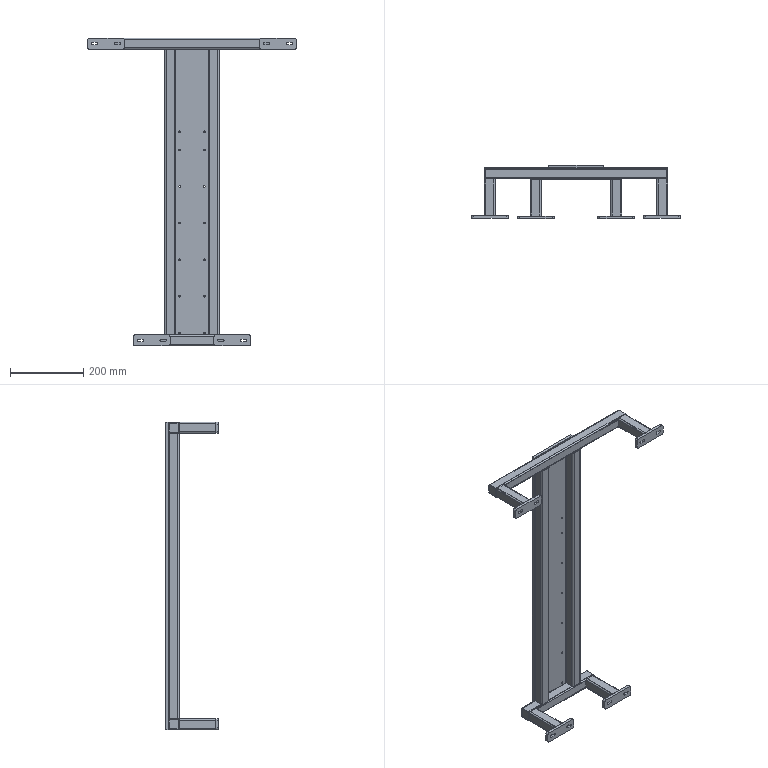Part | SolidWorks | features Fillet 4, ICE 4, 3DProfileFeature 1, EndCap 1, HoleWzd 1, MirrorPattern 1, WeldMemberFeat 1, WeldmentFeature 1 | 17 solids | 274 faces | box 570 x 146 x 840 mm | volume 1678551 mm3 | plane 150 | cylinder 124 | commonest cylinder face diameters 4 x32 8 x32 4.2 x28 7 x16 10 x16